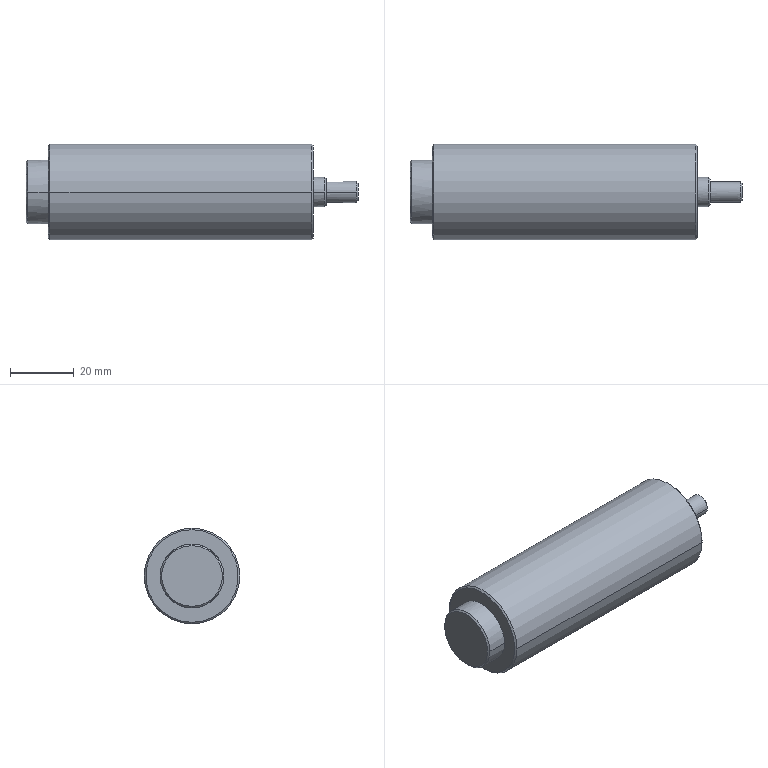Part | SolidWorks | features Chamfer 1, Revolution 1 | 1 solid | 23 faces | box 104 x 30 x 30 mm | volume 61439 mm3 | cone 10 | cylinder 8 | plane 5 | commonest cylinder face diameters 6.6 x2 9.2 x2 20 x2 30 x2
STEP:
#1=CARTESIAN_POINT('',(695.509,27.35,-2.8));
#2=VERTEX_POINT('',#1);
#3=CARTESIAN_POINT('',(695.509,27.35,2.8));
#4=VERTEX_POINT('',#3);
#5=CARTESIAN_POINT('',(695.509,27.35,0.));
#6=DIRECTION('',(1.,0.,0.));
#7=DIRECTION('',(0.,1.,0.));
#8=AXIS2_PLACEMENT_3D('',#5,#6,#7);
#9=CIRCLE('',#8,2.8);
#10=EDGE_CURVE('',#2,#4,#9,.T.);
#11=ORIENTED_EDGE('',*,*,#10,.F.);
#12=CARTESIAN_POINT('',(695.009,27.35,-3.3));
#13=VERTEX_POINT('',#12);
#14=CARTESIAN_POINT('',(695.509,27.35,-2.8));
#15=DIRECTION('',(-0.7071,0.,-0.7071));
#16=VECTOR('',#15,1000.);
#17=LINE('',#14,#16);
#18=EDGE_CURVE('',#2,#13,#17,.T.);
#19=ORIENTED_EDGE('',*,*,#18,.T.);
#20=CARTESIAN_POINT('',(695.009,30.65,0.));
#21=VERTEX_POINT('',#20);
#22=CARTESIAN_POINT('',(695.009,27.35,0.));
#23=DIRECTION('',(-1.,0.,0.));
#24=DIRECTION('',(0.,0.,-1.));
#25=AXIS2_PLACEMENT_3D('',#22,#23,#24);
#26=CIRCLE('',#25,3.3);
#27=EDGE_CURVE('',#21,#13,#26,.T.);
#28=ORIENTED_EDGE('',*,*,#27,.F.);
#29=CARTESIAN_POINT('',(695.009,27.35,3.3));
#30=VERTEX_POINT('',#29);
#31=CARTESIAN_POINT('',(695.009,27.35,0.));
#32=DIRECTION('',(-1.,0.,0.));
#33=DIRECTION('',(0.,0.,-1.));
#34=AXIS2_PLACEMENT_3D('',#31,#32,#33);
#35=CIRCLE('',#34,3.3);
#36=EDGE_CURVE('',#30,#21,#35,.T.);
#37=ORIENTED_EDGE('',*,*,#36,.F.);
#38=CARTESIAN_POINT('',(695.509,27.35,2.8));
#39=DIRECTION('',(-0.7071,0.,0.7071));
#40=VECTOR('',#39,1000.);
#41=LINE('',#38,#40);
#42=EDGE_CURVE('',#4,#30,#41,.T.);
#43=ORIENTED_EDGE('',*,*,#42,.F.);
#44=EDGE_LOOP('',(#11,#19,#28,#37,#43));
#45=FACE_OUTER_BOUND('',#44,.T.);
#46=CARTESIAN_POINT('',(695.509,27.35,0.));
#47=DIRECTION('',(-1.,0.,0.));
#48=DIRECTION('',(0.,0.,1.));
#49=AXIS2_PLACEMENT_3D('',#46,#47,#48);
#50=CONICAL_SURFACE('',#49,2.8,0.7854);
#51=ADVANCED_FACE('',(#45),#50,.T.);
#52=CARTESIAN_POINT('',(685.509,27.35,-4.1));
#53=VERTEX_POINT('',#52);
#54=CARTESIAN_POINT('',(685.509,27.35,4.1));
#55=VERTEX_POINT('',#54);
#56=CARTESIAN_POINT('',(685.509,27.35,0.));
#57=DIRECTION('',(1.,0.,0.));
#58=DIRECTION('',(0.,1.,0.));
#59=AXIS2_PLACEMENT_3D('',#56,#57,#58);
#60=CIRCLE('',#59,4.1);
#61=EDGE_CURVE('',#53,#55,#60,.T.);
#62=ORIENTED_EDGE('',*,*,#61,.F.);
#63=CARTESIAN_POINT('',(685.009,27.35,-4.6));
#64=VERTEX_POINT('',#63);
#65=CARTESIAN_POINT('',(685.509,27.35,-4.1));
#66=DIRECTION('',(-0.7071,0.,-0.7071));
#67=VECTOR('',#66,1000.);
#68=LINE('',#65,#67);
#69=EDGE_CURVE('',#53,#64,#68,.T.);
#70=ORIENTED_EDGE('',*,*,#69,.T.);
#71=CARTESIAN_POINT('',(685.009,31.95,0.));
#72=VERTEX_POINT('',#71);
#73=CARTESIAN_POINT('',(685.009,27.35,0.));
#74=DIRECTION('',(-1.,0.,0.));
#75=DIRECTION('',(0.,0.,-1.));
#76=AXIS2_PLACEMENT_3D('',#73,#74,#75);
#77=CIRCLE('',#76,4.6);
#78=EDGE_CURVE('',#72,#64,#77,.T.);
#79=ORIENTED_EDGE('',*,*,#78,.F.);
#80=CARTESIAN_POINT('',(685.009,27.35,4.6));
#81=VERTEX_POINT('',#80);
#82=CARTESIAN_POINT('',(685.009,27.35,0.));
#83=DIRECTION('',(-1.,0.,0.));
#84=DIRECTION('',(0.,0.,-1.));
#85=AXIS2_PLACEMENT_3D('',#82,#83,#84);
#86=CIRCLE('',#85,4.6);
#87=EDGE_CURVE('',#81,#72,#86,.T.);
#88=ORIENTED_EDGE('',*,*,#87,.F.);
#89=CARTESIAN_POINT('',(685.509,27.35,4.1));
#90=DIRECTION('',(-0.7071,0.,0.7071));
#91=VECTOR('',#90,1000.);
#92=LINE('',#89,#91);
#93=EDGE_CURVE('',#55,#81,#92,.T.);
#94=ORIENTED_EDGE('',*,*,#93,.F.);
#95=EDGE_LOOP('',(#62,#70,#79,#88,#94));
#96=FACE_OUTER_BOUND('',#95,.T.);
#97=CARTESIAN_POINT('',(685.509,27.35,0.));
#98=DIRECTION('',(-1.,0.,0.));
#99=DIRECTION('',(0.,0.,1.));
#100=AXIS2_PLACEMENT_3D('',#97,#98,#99);
#101=CONICAL_SURFACE('',#100,4.1,0.7854);
#102=ADVANCED_FACE('',(#96),#101,.T.);
#103=CARTESIAN_POINT('',(681.509,27.35,-14.5));
#104=VERTEX_POINT('',#103);
#105=CARTESIAN_POINT('',(681.509,27.35,14.5));
#106=VERTEX_POINT('',#105);
#107=CARTESIAN_POINT('',(681.509,27.35,0.));
#108=DIRECTION('',(1.,0.,0.));
#109=DIRECTION('',(0.,1.,0.));
#110=AXIS2_PLACEMENT_3D('',#107,#108,#109);
#111=CIRCLE('',#110,14.5);
#112=EDGE_CURVE('',#104,#106,#111,.T.);
#113=ORIENTED_EDGE('',*,*,#112,.F.);
#114=CARTESIAN_POINT('',(681.009,27.35,-15.));
#115=VERTEX_POINT('',#114);
#116=CARTESIAN_POINT('',(681.509,27.35,-14.5));
#117=DIRECTION('',(-0.7071,0.,-0.7071));
#118=VECTOR('',#117,1000.);
#119=LINE('',#116,#118);
#120=EDGE_CURVE('',#104,#115,#119,.T.);
#121=ORIENTED_EDGE('',*,*,#120,.T.);
#122=CARTESIAN_POINT('',(681.009,42.35,0.));
#123=VERTEX_POINT('',#122);
#124=CARTESIAN_POINT('',(681.009,27.35,0.));
#125=DIRECTION('',(-1.,0.,0.));
#126=DIRECTION('',(0.,0.,-1.));
#127=AXIS2_PLACEMENT_3D('',#124,#125,#126);
#128=CIRCLE('',#127,15.);
#129=EDGE_CURVE('',#123,#115,#128,.T.);
#130=ORIENTED_EDGE('',*,*,#129,.F.);
#131=CARTESIAN_POINT('',(681.009,27.35,15.));
#132=VERTEX_POINT('',#131);
#133=CARTESIAN_POINT('',(681.009,27.35,0.));
#134=DIRECTION('',(-1.,0.,0.));
#135=DIRECTION('',(0.,0.,-1.));
#136=AXIS2_PLACEMENT_3D('',#133,#134,#135);
#137=CIRCLE('',#136,15.);
#138=EDGE_CURVE('',#132,#123,#137,.T.);
#139=ORIENTED_EDGE('',*,*,#138,.F.);
#140=CARTESIAN_POINT('',(681.509,27.35,14.5));
#141=DIRECTION('',(-0.7071,0.,0.7071));
#142=VECTOR('',#141,1000.);
#143=LINE('',#140,#142);
#144=EDGE_CURVE('',#106,#132,#143,.T.);
#145=ORIENTED_EDGE('',*,*,#144,.F.);
#146=EDGE_LOOP('',(#113,#121,#130,#139,#145));
#147=FACE_OUTER_BOUND('',#146,.T.);
#148=CARTESIAN_POINT('',(681.509,27.35,0.));
#149=DIRECTION('',(-1.,0.,0.));
#150=DIRECTION('',(0.,0.,1.));
#151=AXIS2_PLACEMENT_3D('',#148,#149,#150);
#152=CONICAL_SURFACE('',#151,14.5,0.7854);
#153=ADVANCED_FACE('',(#147),#152,.T.);
#154=CARTESIAN_POINT('',(598.509,27.35,14.5));
#155=VERTEX_POINT('',#154);
#156=CARTESIAN_POINT('',(598.509,27.35,-14.5));
#157=VERTEX_POINT('',#156);
#158=CARTESIAN_POINT('',(598.509,27.35,0.));
#159=DIRECTION('',(-1.,0.,0.));
#160=DIRECTION('',(0.,-1.,0.));
#161=AXIS2_PLACEMENT_3D('',#158,#159,#160);
#162=CIRCLE('',#161,14.5);
#163=EDGE_CURVE('',#155,#157,#162,.T.);
#164=ORIENTED_EDGE('',*,*,#163,.F.);
#165=CARTESIAN_POINT('',(599.009,27.35,15.));
#166=VERTEX_POINT('',#165);
#167=CARTESIAN_POINT('',(599.009,27.35,15.));
#168=DIRECTION('',(0.7071,0.,0.7071));
#169=VECTOR('',#168,1000.);
#170=LINE('',#167,#169);
#171=EDGE_CURVE('',#155,#166,#170,.T.);
#172=ORIENTED_EDGE('',*,*,#171,.T.);
#173=CARTESIAN_POINT('',(599.009,42.35,0.));
#174=VERTEX_POINT('',#173);
#175=CARTESIAN_POINT('',(599.009,27.35,0.));
#176=DIRECTION('',(1.,0.,0.));
#177=DIRECTION('',(0.,0.,1.));
#178=AXIS2_PLACEMENT_3D('',#175,#176,#177);
#179=CIRCLE('',#178,15.);
#180=EDGE_CURVE('',#174,#166,#179,.T.);
#181=ORIENTED_EDGE('',*,*,#180,.F.);
#182=CARTESIAN_POINT('',(599.009,27.35,-15.));
#183=VERTEX_POINT('',#182);
#184=CARTESIAN_POINT('',(599.009,27.35,0.));
#185=DIRECTION('',(1.,0.,0.));
#186=DIRECTION('',(0.,0.,1.));
#187=AXIS2_PLACEMENT_3D('',#184,#185,#186);
#188=CIRCLE('',#187,15.);
#189=EDGE_CURVE('',#183,#174,#188,.T.);
#190=ORIENTED_EDGE('',*,*,#189,.F.);
#191=CARTESIAN_POINT('',(599.009,27.35,-15.));
#192=DIRECTION('',(0.7071,0.,-0.7071));
#193=VECTOR('',#192,1000.);
#194=LINE('',#191,#193);
#195=EDGE_CURVE('',#157,#183,#194,.T.);
#196=ORIENTED_EDGE('',*,*,#195,.F.);
#197=EDGE_LOOP('',(#164,#172,#181,#190,#196));
#198=FACE_OUTER_BOUND('',#197,.T.);
#199=CARTESIAN_POINT('',(599.009,27.35,0.));
#200=DIRECTION('',(1.,0.,0.));
#201=DIRECTION('',(0.,0.,-1.));
#202=AXIS2_PLACEMENT_3D('',#199,#200,#201);
#203=CONICAL_SURFACE('',#202,15.,0.7854);
#204=ADVANCED_FACE('',(#198),#203,.T.);
#205=CARTESIAN_POINT('',(591.509,27.35,9.5));
#206=VERTEX_POINT('',#205);
#207=CARTESIAN_POINT('',(591.509,27.35,-9.5));
#208=VERTEX_POINT('',#207);
#209=CARTESIAN_POINT('',(591.509,27.35,0.));
#210=DIRECTION('',(-1.,0.,0.));
#211=DIRECTION('',(0.,-1.,0.));
#212=AXIS2_PLACEMENT_3D('',#209,#210,#211);
#213=CIRCLE('',#212,9.5);
#214=EDGE_CURVE('',#206,#208,#213,.T.);
#215=ORIENTED_EDGE('',*,*,#214,.F.);
#216=CARTESIAN_POINT('',(592.009,27.35,10.));
#217=VERTEX_POINT('',#216);
#218=CARTESIAN_POINT('',(592.009,27.35,10.));
#219=DIRECTION('',(0.7071,0.,0.7071));
#220=VECTOR('',#219,1000.);
#221=LINE('',#218,#220);
#222=EDGE_CURVE('',#206,#217,#221,.T.);
#223=ORIENTED_EDGE('',*,*,#222,.T.);
#224=CARTESIAN_POINT('',(592.009,37.35,0.));
#225=VERTEX_POINT('',#224);
#226=CARTESIAN_POINT('',(592.009,27.35,0.));
#227=DIRECTION('',(1.,0.,0.));
#228=DIRECTION('',(0.,0.,1.));
#229=AXIS2_PLACEMENT_3D('',#226,#227,#228);
#230=CIRCLE('',#229,10.);
#231=EDGE_CURVE('',#225,#217,#230,.T.);
#232=ORIENTED_EDGE('',*,*,#231,.F.);
#233=CARTESIAN_POINT('',(592.009,27.35,-10.));
#234=VERTEX_POINT('',#233);
#235=CARTESIAN_POINT('',(592.009,27.35,0.));
#236=DIRECTION('',(1.,0.,0.));
#237=DIRECTION('',(0.,0.,1.));
#238=AXIS2_PLACEMENT_3D('',#235,#236,#237);
#239=CIRCLE('',#238,10.);
#240=EDGE_CURVE('',#234,#225,#239,.T.);
#241=ORIENTED_EDGE('',*,*,#240,.F.);
#242=CARTESIAN_POINT('',(592.009,27.35,-10.));
#243=DIRECTION('',(0.7071,0.,-0.7071));
#244=VECTOR('',#243,1000.);
#245=LINE('',#242,#244);
#246=EDGE_CURVE('',#208,#234,#245,.T.);
#247=ORIENTED_EDGE('',*,*,#246,.F.);
#248=EDGE_LOOP('',(#215,#223,#232,#241,#247));
#249=FACE_OUTER_BOUND('',#248,.T.);
#250=CARTESIAN_POINT('',(592.009,27.35,0.));
#251=DIRECTION('',(1.,0.,0.));
#252=DIRECTION('',(0.,0.,-1.));
#253=AXIS2_PLACEMENT_3D('',#250,#251,#252);
#254=CONICAL_SURFACE('',#253,10.,0.7854);
#255=ADVANCED_FACE('',(#249),#254,.T.);
#256=ORIENTED_EDGE('',*,*,#180,.T.);
#257=CARTESIAN_POINT('',(599.009,12.35,0.));
#258=VERTEX_POINT('',#257);
#259=CARTESIAN_POINT('',(599.009,27.35,0.));
#260=DIRECTION('',(1.,0.,0.));
#261=DIRECTION('',(0.,0.,1.));
#262=AXIS2_PLACEMENT_3D('',#259,#260,#261);
#263=CIRCLE('',#262,15.);
#264=EDGE_CURVE('',#166,#258,#263,.T.);
#265=ORIENTED_EDGE('',*,*,#264,.T.);
#266=CARTESIAN_POINT('',(681.009,12.35,0.));
#267=VERTEX_POINT('',#266);
#268=CARTESIAN_POINT('',(695.509,12.35,0.));
#269=DIRECTION('',(1.,0.,0.));
#270=VECTOR('',#269,1000.);
#271=LINE('',#268,#270);
#272=EDGE_CURVE('',#258,#267,#271,.T.);
#273=ORIENTED_EDGE('',*,*,#272,.T.);
#274=CARTESIAN_POINT('',(681.009,27.35,0.));
#275=DIRECTION('',(-1.,0.,0.));
#276=DIRECTION('',(0.,0.,-1.));
#277=AXIS2_PLACEMENT_3D('',#274,#275,#276);
#278=CIRCLE('',#277,15.);
#279=EDGE_CURVE('',#267,#132,#278,.T.);
#280=ORIENTED_EDGE('',*,*,#279,.T.);
#281=ORIENTED_EDGE('',*,*,#138,.T.);
#282=CARTESIAN_POINT('',(695.509,42.35,0.));
#283=DIRECTION('',(1.,0.,0.));
#284=VECTOR('',#283,1000.);
#285=LINE('',#282,#284);
#286=EDGE_CURVE('',#174,#123,#285,.T.);
#287=ORIENTED_EDGE('',*,*,#286,.F.);
#288=EDGE_LOOP('',(#256,#265,#273,#280,#281,#287));
#289=FACE_OUTER_BOUND('',#288,.T.);
#290=CARTESIAN_POINT('',(695.509,27.35,0.));
#291=DIRECTION('',(1.,0.,0.));
#292=DIRECTION('',(0.,1.,0.));
#293=AXIS2_PLACEMENT_3D('',#290,#291,#292);
#294=CYLINDRICAL_SURFACE('',#293,15.);
#295=ADVANCED_FACE('',(#289),#294,.T.);
#296=ORIENTED_EDGE('',*,*,#231,.T.);
#297=CARTESIAN_POINT('',(592.009,17.35,0.));
#298=VERTEX_POINT('',#297);
#299=CARTESIAN_POINT('',(592.009,27.35,0.));
#300=DIRECTION('',(1.,0.,0.));
#301=DIRECTION('',(0.,0.,1.));
#302=AXIS2_PLACEMENT_3D('',#299,#300,#301);
#303=CIRCLE('',#302,10.);
#304=EDGE_CURVE('',#217,#298,#303,.T.);
#305=ORIENTED_EDGE('',*,*,#304,.T.);
#306=CARTESIAN_POINT('',(598.509,17.35,0.));
#307=VERTEX_POINT('',#306);
#308=CARTESIAN_POINT('',(695.509,17.35,0.));
#309=DIRECTION('',(1.,0.,0.));
#310=VECTOR('',#309,1000.);
#311=LINE('',#308,#310);
#312=EDGE_CURVE('',#298,#307,#311,.T.);
#313=ORIENTED_EDGE('',*,*,#312,.T.);
#314=CARTESIAN_POINT('',(598.509,37.35,0.));
#315=VERTEX_POINT('',#314);
#316=CARTESIAN_POINT('',(598.509,27.35,0.));
#317=DIRECTION('',(1.,0.,0.));
#318=DIRECTION('',(0.,1.,0.));
#319=AXIS2_PLACEMENT_3D('',#316,#317,#318);
#320=CIRCLE('',#319,10.);
#321=EDGE_CURVE('',#315,#307,#320,.T.);
#322=ORIENTED_EDGE('',*,*,#321,.F.);
#323=CARTESIAN_POINT('',(695.509,37.35,0.));
#324=DIRECTION('',(1.,0.,0.));
#325=VECTOR('',#324,1000.);
#326=LINE('',#323,#325);
#327=EDGE_CURVE('',#225,#315,#326,.T.);
#328=ORIENTED_EDGE('',*,*,#327,.F.);
#329=EDGE_LOOP('',(#296,#305,#313,#322,#328));
#330=FACE_OUTER_BOUND('',#329,.T.);
#331=CARTESIAN_POINT('',(695.509,27.35,0.));
#332=DIRECTION('',(1.,0.,0.));
#333=DIRECTION('',(0.,1.,0.));
#334=AXIS2_PLACEMENT_3D('',#331,#332,#333);
#335=CYLINDRICAL_SURFACE('',#334,10.);
#336=ADVANCED_FACE('',(#330),#335,.T.);
#337=CARTESIAN_POINT('',(685.509,30.65,0.));
#338=VERTEX_POINT('',#337);
#339=CARTESIAN_POINT('',(685.509,24.05,0.));
#340=VERTEX_POINT('',#339);
#341=CARTESIAN_POINT('',(685.509,27.35,0.));
#342=DIRECTION('',(1.,0.,0.));
#343=DIRECTION('',(0.,1.,0.));
#344=AXIS2_PLACEMENT_3D('',#341,#342,#343);
#345=CIRCLE('',#344,3.3);
#346=EDGE_CURVE('',#338,#340,#345,.T.);
#347=ORIENTED_EDGE('',*,*,#346,.T.);
#348=CARTESIAN_POINT('',(695.009,24.05,0.));
#349=VERTEX_POINT('',#348);
#350=CARTESIAN_POINT('',(695.509,24.05,0.));
#351=DIRECTION('',(1.,0.,0.));
#352=VECTOR('',#351,1000.);
#353=LINE('',#350,#352);
#354=EDGE_CURVE('',#340,#349,#353,.T.);
#355=ORIENTED_EDGE('',*,*,#354,.T.);
#356=CARTESIAN_POINT('',(695.009,27.35,0.));
#357=DIRECTION('',(-1.,0.,0.));
#358=DIRECTION('',(0.,0.,-1.));
#359=AXIS2_PLACEMENT_3D('',#356,#357,#358);
#360=CIRCLE('',#359,3.3);
#361=EDGE_CURVE('',#349,#30,#360,.T.);
#362=ORIENTED_EDGE('',*,*,#361,.T.);
#363=ORIENTED_EDGE('',*,*,#36,.T.);
#364=CARTESIAN_POINT('',(695.509,30.65,0.));
#365=DIRECTION('',(1.,0.,0.));
#366=VECTOR('',#365,1000.);
#367=LINE('',#364,#366);
#368=EDGE_CURVE('',#338,#21,#367,.T.);
#369=ORIENTED_EDGE('',*,*,#368,.F.);
#370=EDGE_LOOP('',(#347,#355,#362,#363,#369));
#371=FACE_OUTER_BOUND('',#370,.T.);
#372=CARTESIAN_POINT('',(695.509,27.35,0.));
#373=DIRECTION('',(1.,0.,0.));
#374=DIRECTION('',(0.,1.,0.));
#375=AXIS2_PLACEMENT_3D('',#372,#373,#374);
#376=CYLINDRICAL_SURFACE('',#375,3.3);
#377=ADVANCED_FACE('',(#371),#376,.T.);
#378=CARTESIAN_POINT('',(681.509,31.95,0.));
#379=VERTEX_POINT('',#378);
#380=CARTESIAN_POINT('',(681.509,22.75,0.));
#381=VERTEX_POINT('',#380);
#382=CARTESIAN_POINT('',(681.509,27.35,0.));
#383=DIRECTION('',(1.,0.,0.));
#384=DIRECTION('',(0.,1.,0.));
#385=AXIS2_PLACEMENT_3D('',#382,#383,#384);
#386=CIRCLE('',#385,4.6);
#387=EDGE_CURVE('',#379,#381,#386,.T.);
#388=ORIENTED_EDGE('',*,*,#387,.T.);
#389=CARTESIAN_POINT('',(685.009,22.75,0.));
#390=VERTEX_POINT('',#389);
#391=CARTESIAN_POINT('',(695.509,22.75,0.));
#392=DIRECTION('',(1.,0.,0.));
#393=VECTOR('',#392,1000.);
#394=LINE('',#391,#393);
#395=EDGE_CURVE('',#381,#390,#394,.T.);
#396=ORIENTED_EDGE('',*,*,#395,.T.);
#397=CARTESIAN_POINT('',(685.009,27.35,0.));
#398=DIRECTION('',(-1.,0.,0.));
#399=DIRECTION('',(0.,0.,-1.));
#400=AXIS2_PLACEMENT_3D('',#397,#398,#399);
#401=CIRCLE('',#400,4.6);
#402=EDGE_CURVE('',#390,#81,#401,.T.);
#403=ORIENTED_EDGE('',*,*,#402,.T.);
#404=ORIENTED_EDGE('',*,*,#87,.T.);
#405=CARTESIAN_POINT('',(695.509,31.95,0.));
#406=DIRECTION('',(1.,0.,0.));
#407=VECTOR('',#406,1000.);
#408=LINE('',#405,#407);
#409=EDGE_CURVE('',#379,#72,#408,.T.);
#410=ORIENTED_EDGE('',*,*,#409,.F.);
#411=EDGE_LOOP('',(#388,#396,#403,#404,#410));
#412=FACE_OUTER_BOUND('',#411,.T.);
#413=CARTESIAN_POINT('',(695.509,27.35,0.));
#414=DIRECTION('',(1.,0.,0.));
#415=DIRECTION('',(0.,1.,0.));
#416=AXIS2_PLACEMENT_3D('',#413,#414,#415);
#417=CYLINDRICAL_SURFACE('',#416,4.6);
#418=ADVANCED_FACE('',(#412),#417,.T.);
#419=ORIENTED_EDGE('',*,*,#395,.F.);
#420=CARTESIAN_POINT('',(681.509,27.35,0.));
#421=DIRECTION('',(1.,0.,0.));
#422=DIRECTION('',(0.,1.,0.));
#423=AXIS2_PLACEMENT_3D('',#420,#421,#422);
#424=CIRCLE('',#423,4.6);
#425=EDGE_CURVE('',#381,#379,#424,.T.);
#426=ORIENTED_EDGE('',*,*,#425,.T.);
#427=ORIENTED_EDGE('',*,*,#409,.T.);
#428=ORIENTED_EDGE('',*,*,#78,.T.);
#429=CARTESIAN_POINT('',(685.009,27.35,0.));
#430=DIRECTION('',(-1.,0.,0.));
#431=DIRECTION('',(0.,0.,-1.));
#432=AXIS2_PLACEMENT_3D('',#429,#430,#431);
#433=CIRCLE('',#432,4.6);
#434=EDGE_CURVE('',#64,#390,#433,.T.);
#435=ORIENTED_EDGE('',*,*,#434,.T.);
#436=EDGE_LOOP('',(#419,#426,#427,#428,#435));
#437=FACE_OUTER_BOUND('',#436,.T.);
#438=CARTESIAN_POINT('',(695.509,27.35,0.));
#439=DIRECTION('',(1.,0.,0.));
#440=DIRECTION('',(0.,1.,0.));
#441=AXIS2_PLACEMENT_3D('',#438,#439,#440);
#442=CYLINDRICAL_SURFACE('',#441,4.6);
#443=ADVANCED_FACE('',(#437),#442,.T.);
#444=CARTESIAN_POINT('',(685.509,27.35,0.));
#445=DIRECTION('',(1.,0.,0.));
#446=DIRECTION('',(0.,1.,0.));
#447=AXIS2_PLACEMENT_3D('',#444,#445,#446);
#448=CIRCLE('',#447,4.1);
#449=EDGE_CURVE('',#55,#53,#448,.T.);
#450=ORIENTED_EDGE('',*,*,#449,.T.);
#451=ORIENTED_EDGE('',*,*,#61,.T.);
#452=EDGE_LOOP('',(#450,#451));
#453=FACE_OUTER_BOUND('',#452,.T.);
#454=ORIENTED_EDGE('',*,*,#346,.F.);
#455=CARTESIAN_POINT('',(685.509,27.35,0.));
#456=DIRECTION('',(1.,0.,0.));
#457=DIRECTION('',(0.,1.,0.));
#458=AXIS2_PLACEMENT_3D('',#455,#456,#457);
#459=CIRCLE('',#458,3.3);
#460=EDGE_CURVE('',#340,#338,#459,.T.);
#461=ORIENTED_EDGE('',*,*,#460,.F.);
#462=EDGE_LOOP('',(#454,#461));
#463=FACE_BOUND('',#462,.T.);
#464=CARTESIAN_POINT('',(685.509,30.65,0.));
#465=DIRECTION('',(1.,0.,0.));
#466=DIRECTION('',(0.,1.,0.));
#467=AXIS2_PLACEMENT_3D('',#464,#465,#466);
#468=PLANE('',#467);
#469=ADVANCED_FACE('',(#453,#463),#468,.T.);
#470=ORIENTED_EDGE('',*,*,#354,.F.);
#471=ORIENTED_EDGE('',*,*,#460,.T.);
#472=ORIENTED_EDGE('',*,*,#368,.T.);
#473=ORIENTED_EDGE('',*,*,#27,.T.);
#474=CARTESIAN_POINT('',(695.009,27.35,0.));
#475=DIRECTION('',(-1.,0.,0.));
#476=DIRECTION('',(0.,0.,-1.));
#477=AXIS2_PLACEMENT_3D('',#474,#475,#476);
#478=CIRCLE('',#477,3.3);
#479=EDGE_CURVE('',#13,#349,#478,.T.);
#480=ORIENTED_EDGE('',*,*,#479,.T.);
#481=EDGE_LOOP('',(#470,#471,#472,#473,#480));
#482=FACE_OUTER_BOUND('',#481,.T.);
#483=CARTESIAN_POINT('',(695.509,27.35,0.));
#484=DIRECTION('',(1.,0.,0.));
#485=DIRECTION('',(0.,1.,0.));
#486=AXIS2_PLACEMENT_3D('',#483,#484,#485);
#487=CYLINDRICAL_SURFACE('',#486,3.3);
#488=ADVANCED_FACE('',(#482),#487,.T.);
#489=CARTESIAN_POINT('',(695.509,27.35,0.));
#490=DIRECTION('',(1.,0.,0.));
#491=DIRECTION('',(0.,1.,0.));
#492=AXIS2_PLACEMENT_3D('',#489,#490,#491);
#493=CIRCLE('',#492,2.8);
#494=EDGE_CURVE('',#4,#2,#493,.T.);
#495=ORIENTED_EDGE('',*,*,#494,.T.);
#496=ORIENTED_EDGE('',*,*,#10,.T.);
#497=EDGE_LOOP('',(#495,#496));
#498=FACE_OUTER_BOUND('',#497,.T.);
#499=CARTESIAN_POINT('',(695.509,30.65,0.));
#500=DIRECTION('',(1.,0.,0.));
#501=DIRECTION('',(0.,1.,0.));
#502=AXIS2_PLACEMENT_3D('',#499,#500,#501);
#503=PLANE('',#502);
#504=ADVANCED_FACE('',(#498),#503,.T.);
#505=CARTESIAN_POINT('',(591.509,27.35,0.));
#506=DIRECTION('',(-1.,0.,0.));
#507=DIRECTION('',(0.,-1.,0.));
#508=AXIS2_PLACEMENT_3D('',#505,#506,#507);
#509=CIRCLE('',#508,9.5);
#510=EDGE_CURVE('',#208,#206,#509,.T.);
#511=ORIENTED_EDGE('',*,*,#510,.T.);
#512=ORIENTED_EDGE('',*,*,#214,.T.);
#513=EDGE_LOOP('',(#511,#512));
#514=FACE_OUTER_BOUND('',#513,.T.);
#515=CARTESIAN_POINT('',(591.509,37.35,0.));
#516=DIRECTION('',(-1.,0.,0.));
#517=DIRECTION('',(0.,-1.,0.));
#518=AXIS2_PLACEMENT_3D('',#515,#516,#517);
#519=PLANE('',#518);
#520=ADVANCED_FACE('',(#514),#519,.T.);
#521=ORIENTED_EDGE('',*,*,#312,.F.);
#522=CARTESIAN_POINT('',(592.009,27.35,0.));
#523=DIRECTION('',(1.,0.,0.));
#524=DIRECTION('',(0.,0.,1.));
#525=AXIS2_PLACEMENT_3D('',#522,#523,#524);
#526=CIRCLE('',#525,10.);
#527=EDGE_CURVE('',#298,#234,#526,.T.);
#528=ORIENTED_EDGE('',*,*,#527,.T.);
#529=ORIENTED_EDGE('',*,*,#240,.T.);
#530=ORIENTED_EDGE('',*,*,#327,.T.);
#531=CARTESIAN_POINT('',(598.509,27.35,0.));
#532=DIRECTION('',(1.,0.,0.));
#533=DIRECTION('',(0.,1.,0.));
#534=AXIS2_PLACEMENT_3D('',#531,#532,#533);
#535=CIRCLE('',#534,10.);
#536=EDGE_CURVE('',#307,#315,#535,.T.);
#537=ORIENTED_EDGE('',*,*,#536,.F.);
#538=EDGE_LOOP('',(#521,#528,#529,#530,#537));
#539=FACE_OUTER_BOUND('',#538,.T.);
#540=CARTESIAN_POINT('',(695.509,27.35,0.));
#541=DIRECTION('',(1.,0.,0.));
#542=DIRECTION('',(0.,1.,0.));
#543=AXIS2_PLACEMENT_3D('',#540,#541,#542);
#544=CYLINDRICAL_SURFACE('',#543,10.);
#545=ADVANCED_FACE('',(#539),#544,.T.);
#546=CARTESIAN_POINT('',(598.509,27.35,0.));
#547=DIRECTION('',(-1.,0.,0.));
#548=DIRECTION('',(0.,-1.,0.));
#549=AXIS2_PLACEMENT_3D('',#546,#547,#548);
#550=CIRCLE('',#549,14.5);
#551=EDGE_CURVE('',#157,#155,#550,.T.);
#552=ORIENTED_EDGE('',*,*,#551,.T.);
#553=ORIENTED_EDGE('',*,*,#163,.T.);
#554=EDGE_LOOP('',(#552,#553));
#555=FACE_OUTER_BOUND('',#554,.T.);
#556=ORIENTED_EDGE('',*,*,#321,.T.);
#557=ORIENTED_EDGE('',*,*,#536,.T.);
#558=EDGE_LOOP('',(#556,#557));
#559=FACE_BOUND('',#558,.T.);
#560=CARTESIAN_POINT('',(598.509,42.35,0.));
#561=DIRECTION('',(-1.,0.,0.));
#562=DIRECTION('',(0.,-1.,0.));
#563=AXIS2_PLACEMENT_3D('',#560,#561,#562);
#564=PLANE('',#563);
#565=ADVANCED_FACE('',(#555,#559),#564,.T.);
#566=ORIENTED_EDGE('',*,*,#272,.F.);
#567=CARTESIAN_POINT('',(599.009,27.35,0.));
#568=DIRECTION('',(1.,0.,0.));
#569=DIRECTION('',(0.,0.,1.));
#570=AXIS2_PLACEMENT_3D('',#567,#568,#569);
#571=CIRCLE('',#570,15.);
#572=EDGE_CURVE('',#258,#183,#571,.T.);
#573=ORIENTED_EDGE('',*,*,#572,.T.);
#574=ORIENTED_EDGE('',*,*,#189,.T.);
#575=ORIENTED_EDGE('',*,*,#286,.T.);
#576=ORIENTED_EDGE('',*,*,#129,.T.);
#577=CARTESIAN_POINT('',(681.009,27.35,0.));
#578=DIRECTION('',(-1.,0.,0.));
#579=DIRECTION('',(0.,0.,-1.));
#580=AXIS2_PLACEMENT_3D('',#577,#578,#579);
#581=CIRCLE('',#580,15.);
#582=EDGE_CURVE('',#115,#267,#581,.T.);
#583=ORIENTED_EDGE('',*,*,#582,.T.);
#584=EDGE_LOOP('',(#566,#573,#574,#575,#576,#583));
#585=FACE_OUTER_BOUND('',#584,.T.);
#586=CARTESIAN_POINT('',(695.509,27.35,0.));
#587=DIRECTION('',(1.,0.,0.));
#588=DIRECTION('',(0.,1.,0.));
#589=AXIS2_PLACEMENT_3D('',#586,#587,#588);
#590=CYLINDRICAL_SURFACE('',#589,15.);
#591=ADVANCED_FACE('',(#585),#590,.T.);
#592=CARTESIAN_POINT('',(681.509,27.35,0.));
#593=DIRECTION('',(1.,0.,0.));
#594=DIRECTION('',(0.,1.,0.));
#595=AXIS2_PLACEMENT_3D('',#592,#593,#594);
#596=CIRCLE('',#595,14.5);
#597=EDGE_CURVE('',#106,#104,#596,.T.);
#598=ORIENTED_EDGE('',*,*,#597,.T.);
#599=ORIENTED_EDGE('',*,*,#112,.T.);
#600=EDGE_LOOP('',(#598,#599));
#601=FACE_OUTER_BOUND('',#600,.T.);
#602=ORIENTED_EDGE('',*,*,#387,.F.);
#603=ORIENTED_EDGE('',*,*,#425,.F.);
#604=EDGE_LOOP('',(#602,#603));
#605=FACE_BOUND('',#604,.T.);
#606=CARTESIAN_POINT('',(681.509,31.95,0.));
#607=DIRECTION('',(1.,0.,0.));
#608=DIRECTION('',(0.,1.,0.));
#609=AXIS2_PLACEMENT_3D('',#606,#607,#608);
#610=PLANE('',#609);
#611=ADVANCED_FACE('',(#601,#605),#610,.T.);
#612=ORIENTED_EDGE('',*,*,#222,.F.);
#613=ORIENTED_EDGE('',*,*,#510,.F.);
#614=ORIENTED_EDGE('',*,*,#246,.T.);
#615=ORIENTED_EDGE('',*,*,#527,.F.);
#616=ORIENTED_EDGE('',*,*,#304,.F.);
#617=EDGE_LOOP('',(#612,#613,#614,#615,#616));
#618=FACE_OUTER_BOUND('',#617,.T.);
#619=CARTESIAN_POINT('',(592.009,27.35,0.));
#620=DIRECTION('',(1.,0.,0.));
#621=DIRECTION('',(0.,0.,-1.));
#622=AXIS2_PLACEMENT_3D('',#619,#620,#621);
#623=CONICAL_SURFACE('',#622,10.,0.7854);
#624=ADVANCED_FACE('',(#618),#623,.T.);
#625=ORIENTED_EDGE('',*,*,#171,.F.);
#626=ORIENTED_EDGE('',*,*,#551,.F.);
#627=ORIENTED_EDGE('',*,*,#195,.T.);
#628=ORIENTED_EDGE('',*,*,#572,.F.);
#629=ORIENTED_EDGE('',*,*,#264,.F.);
#630=EDGE_LOOP('',(#625,#626,#627,#628,#629));
#631=FACE_OUTER_BOUND('',#630,.T.);
#632=CARTESIAN_POINT('',(599.009,27.35,0.));
#633=DIRECTION('',(1.,0.,0.));
#634=DIRECTION('',(0.,0.,-1.));
#635=AXIS2_PLACEMENT_3D('',#632,#633,#634);
#636=CONICAL_SURFACE('',#635,15.,0.7854);
#637=ADVANCED_FACE('',(#631),#636,.T.);
#638=ORIENTED_EDGE('',*,*,#120,.F.);
#639=ORIENTED_EDGE('',*,*,#597,.F.);
#640=ORIENTED_EDGE('',*,*,#144,.T.);
#641=ORIENTED_EDGE('',*,*,#279,.F.);
#642=ORIENTED_EDGE('',*,*,#582,.F.);
#643=EDGE_LOOP('',(#638,#639,#640,#641,#642));
#644=FACE_OUTER_BOUND('',#643,.T.);
#645=CARTESIAN_POINT('',(681.509,27.35,0.));
#646=DIRECTION('',(-1.,0.,0.));
#647=DIRECTION('',(0.,0.,1.));
#648=AXIS2_PLACEMENT_3D('',#645,#646,#647);
#649=CONICAL_SURFACE('',#648,14.5,0.7854);
#650=ADVANCED_FACE('',(#644),#649,.T.);
#651=ORIENTED_EDGE('',*,*,#69,.F.);
#652=ORIENTED_EDGE('',*,*,#449,.F.);
#653=ORIENTED_EDGE('',*,*,#93,.T.);
#654=ORIENTED_EDGE('',*,*,#402,.F.);
#655=ORIENTED_EDGE('',*,*,#434,.F.);
#656=EDGE_LOOP('',(#651,#652,#653,#654,#655));
#657=FACE_OUTER_BOUND('',#656,.T.);
#658=CARTESIAN_POINT('',(685.509,27.35,0.));
#659=DIRECTION('',(-1.,0.,0.));
#660=DIRECTION('',(0.,0.,1.));
#661=AXIS2_PLACEMENT_3D('',#658,#659,#660);
#662=CONICAL_SURFACE('',#661,4.1,0.7854);
#663=ADVANCED_FACE('',(#657),#662,.T.);
#664=ORIENTED_EDGE('',*,*,#18,.F.);
#665=ORIENTED_EDGE('',*,*,#494,.F.);
#666=ORIENTED_EDGE('',*,*,#42,.T.);
#667=ORIENTED_EDGE('',*,*,#361,.F.);
#668=ORIENTED_EDGE('',*,*,#479,.F.);
#669=EDGE_LOOP('',(#664,#665,#666,#667,#668));
#670=FACE_OUTER_BOUND('',#669,.T.);
#671=CARTESIAN_POINT('',(695.509,27.35,0.));
#672=DIRECTION('',(-1.,0.,0.));
#673=DIRECTION('',(0.,0.,1.));
#674=AXIS2_PLACEMENT_3D('',#671,#672,#673);
#675=CONICAL_SURFACE('',#674,2.8,0.7854);
#676=ADVANCED_FACE('',(#670),#675,.T.);
#677=CLOSED_SHELL('',(#51,#102,#153,#204,#255,#295,#336,#377,#418,#443,#469,#488,#504,#520,#545,#565,#591,#611,#624,#637,#650,#663,#676));
#678=MANIFOLD_SOLID_BREP('',#677);
#679=CARTESIAN_POINT('',(0.,0.,0.));
#680=DIRECTION('',(0.,0.,1.));
#681=DIRECTION('',(1.,0.,0.));
#682=AXIS2_PLACEMENT_3D('',#679,#680,#681);
#683=(LENGTH_UNIT()NAMED_UNIT(*)SI_UNIT(.MILLI.,.METRE.));
#684=UNCERTAINTY_MEASURE_WITH_UNIT(LENGTH_MEASURE(0.00001),#683,'','');
#685=(NAMED_UNIT(*)PLANE_ANGLE_UNIT()SI_UNIT($,.RADIAN.));
#686=(NAMED_UNIT(*)SI_UNIT($,.STERADIAN.)SOLID_ANGLE_UNIT());
#687=(GEOMETRIC_REPRESENTATION_CONTEXT(3)GLOBAL_UNCERTAINTY_ASSIGNED_CONTEXT((#684))GLOBAL_UNIT_ASSIGNED_CONTEXT((#683,#685,#686))REPRESENTATION_CONTEXT('',''));
#688=ADVANCED_BREP_SHAPE_REPRESENTATION('',(#678,#682),#687);